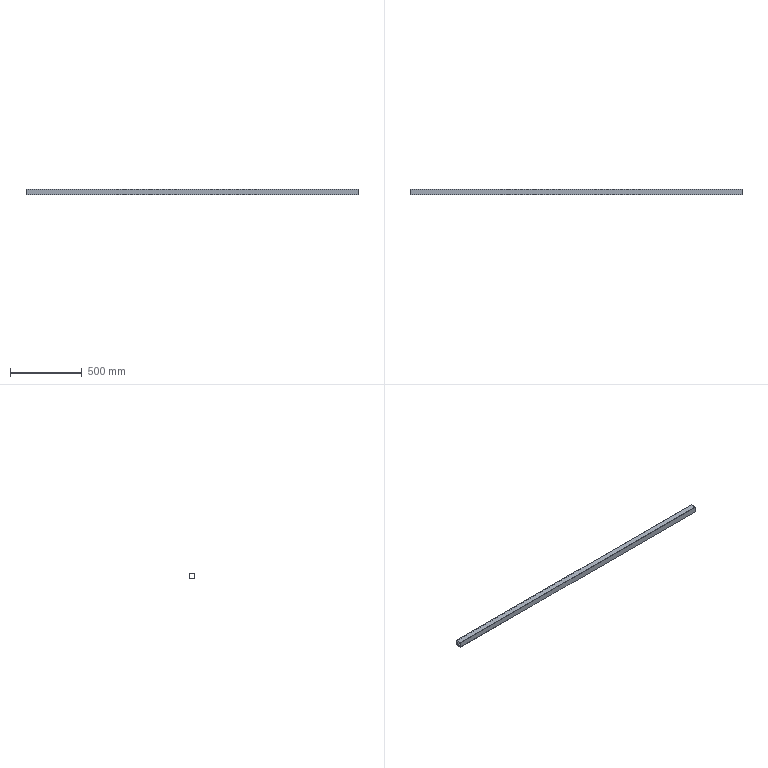Part | NX | features solid 2 | 1 solid | 10 faces | box 2320 x 40 x 40 mm | volume 1336320 mm3 | plane 10
STEP:
#1=CARTESIAN_POINT('',(-1180.,-220.,-45.));
#2=VERTEX_POINT('',#1);
#3=CARTESIAN_POINT('',(1140.,-220.,-45.));
#4=VERTEX_POINT('',#3);
#5=CARTESIAN_POINT('',(204.393,-220.,-45.));
#6=DIRECTION('',(1.,0.,0.));
#7=VECTOR('',#6,1000.);
#8=LINE('',#5,#7);
#9=EDGE_CURVE('',#2,#4,#8,.T.);
#10=ORIENTED_EDGE('',*,*,#9,.F.);
#11=CARTESIAN_POINT('',(-1180.,-220.,-85.));
#12=VERTEX_POINT('',#11);
#13=CARTESIAN_POINT('',(-1180.,-220.,-70.));
#14=DIRECTION('',(0.,0.,-1.));
#15=VECTOR('',#14,1000.);
#16=LINE('',#13,#15);
#17=EDGE_CURVE('',#2,#12,#16,.T.);
#18=ORIENTED_EDGE('',*,*,#17,.T.);
#19=CARTESIAN_POINT('',(1140.,-220.,-85.));
#20=VERTEX_POINT('',#19);
#21=CARTESIAN_POINT('',(119.393,-220.,-85.));
#22=DIRECTION('',(1.,0.,0.));
#23=VECTOR('',#22,1000.);
#24=LINE('',#21,#23);
#25=EDGE_CURVE('',#12,#20,#24,.T.);
#26=ORIENTED_EDGE('',*,*,#25,.T.);
#27=CARTESIAN_POINT('',(1140.,-220.,-70.));
#28=DIRECTION('',(0.,0.,-1.));
#29=VECTOR('',#28,1000.);
#30=LINE('',#27,#29);
#31=EDGE_CURVE('',#4,#20,#30,.T.);
#32=ORIENTED_EDGE('',*,*,#31,.F.);
#33=EDGE_LOOP('',(#10,#18,#26,#32));
#34=FACE_BOUND('',#33,.T.);
#35=CARTESIAN_POINT('',(119.393,-220.,-70.));
#36=DIRECTION('',(0.,1.,0.));
#37=DIRECTION('',(0.,0.,1.));
#38=AXIS2_PLACEMENT_3D('',#35,#36,#37);
#39=PLANE('',#38);
#40=ADVANCED_FACE('',(#34),#39,.F.);
#41=ORIENTED_EDGE('',*,*,#25,.F.);
#42=CARTESIAN_POINT('',(-1180.,-180.,-85.));
#43=VERTEX_POINT('',#42);
#44=CARTESIAN_POINT('',(-1180.,-800.,-85.));
#45=DIRECTION('',(0.,1.,0.));
#46=VECTOR('',#45,1000.);
#47=LINE('',#44,#46);
#48=EDGE_CURVE('',#12,#43,#47,.T.);
#49=ORIENTED_EDGE('',*,*,#48,.T.);
#50=CARTESIAN_POINT('',(1140.,-180.,-85.));
#51=VERTEX_POINT('',#50);
#52=CARTESIAN_POINT('',(204.393,-180.,-85.));
#53=DIRECTION('',(1.,0.,0.));
#54=VECTOR('',#53,1000.);
#55=LINE('',#52,#54);
#56=EDGE_CURVE('',#43,#51,#55,.T.);
#57=ORIENTED_EDGE('',*,*,#56,.T.);
#58=CARTESIAN_POINT('',(1140.,-800.,-85.));
#59=DIRECTION('',(0.,1.,0.));
#60=VECTOR('',#59,1000.);
#61=LINE('',#58,#60);
#62=EDGE_CURVE('',#20,#51,#61,.T.);
#63=ORIENTED_EDGE('',*,*,#62,.F.);
#64=EDGE_LOOP('',(#41,#49,#57,#63));
#65=FACE_BOUND('',#64,.T.);
#66=CARTESIAN_POINT('',(204.393,-800.,-85.));
#67=DIRECTION('',(0.,0.,1.));
#68=DIRECTION('',(0.,-1.,0.));
#69=AXIS2_PLACEMENT_3D('',#66,#67,#68);
#70=PLANE('',#69);
#71=ADVANCED_FACE('',(#65),#70,.F.);
#72=CARTESIAN_POINT('',(1140.,-180.,-45.));
#73=VERTEX_POINT('',#72);
#74=CARTESIAN_POINT('',(-1180.,-180.,-45.));
#75=VERTEX_POINT('',#74);
#76=CARTESIAN_POINT('',(204.393,-180.,-45.));
#77=DIRECTION('',(-1.,0.,0.));
#78=VECTOR('',#77,1000.);
#79=LINE('',#76,#78);
#80=EDGE_CURVE('',#73,#75,#79,.T.);
#81=ORIENTED_EDGE('',*,*,#80,.T.);
#82=CARTESIAN_POINT('',(-1180.,-840.,-45.));
#83=DIRECTION('',(0.,-1.,0.));
#84=VECTOR('',#83,1000.);
#85=LINE('',#82,#84);
#86=EDGE_CURVE('',#75,#2,#85,.T.);
#87=ORIENTED_EDGE('',*,*,#86,.T.);
#88=ORIENTED_EDGE('',*,*,#9,.T.);
#89=CARTESIAN_POINT('',(1140.,-840.,-45.));
#90=DIRECTION('',(0.,-1.,0.));
#91=VECTOR('',#90,1000.);
#92=LINE('',#89,#91);
#93=EDGE_CURVE('',#73,#4,#92,.T.);
#94=ORIENTED_EDGE('',*,*,#93,.F.);
#95=EDGE_LOOP('',(#81,#87,#88,#94));
#96=FACE_BOUND('',#95,.T.);
#97=CARTESIAN_POINT('',(204.393,-840.,-45.));
#98=DIRECTION('',(0.,0.,-1.));
#99=DIRECTION('',(0.,1.,0.));
#100=AXIS2_PLACEMENT_3D('',#97,#98,#99);
#101=PLANE('',#100);
#102=ADVANCED_FACE('',(#96),#101,.F.);
#103=ORIENTED_EDGE('',*,*,#56,.F.);
#104=CARTESIAN_POINT('',(-1180.,-180.,-40.));
#105=DIRECTION('',(0.,0.,1.));
#106=VECTOR('',#105,1000.);
#107=LINE('',#104,#106);
#108=EDGE_CURVE('',#43,#75,#107,.T.);
#109=ORIENTED_EDGE('',*,*,#108,.T.);
#110=ORIENTED_EDGE('',*,*,#80,.F.);
#111=CARTESIAN_POINT('',(1140.,-180.,-40.));
#112=DIRECTION('',(0.,0.,1.));
#113=VECTOR('',#112,1000.);
#114=LINE('',#111,#113);
#115=EDGE_CURVE('',#51,#73,#114,.T.);
#116=ORIENTED_EDGE('',*,*,#115,.F.);
#117=EDGE_LOOP('',(#103,#109,#110,#116));
#118=FACE_BOUND('',#117,.T.);
#119=CARTESIAN_POINT('',(119.393,-180.,-40.));
#120=DIRECTION('',(0.,-1.,0.));
#121=DIRECTION('',(0.,0.,-1.));
#122=AXIS2_PLACEMENT_3D('',#119,#120,#121);
#123=PLANE('',#122);
#124=ADVANCED_FACE('',(#118),#123,.F.);
#125=CARTESIAN_POINT('',(-1180.,-216.,-49.));
#126=VERTEX_POINT('',#125);
#127=CARTESIAN_POINT('',(-1180.,-216.,-81.));
#128=VERTEX_POINT('',#127);
#129=CARTESIAN_POINT('',(-1180.,-216.,-70.));
#130=DIRECTION('',(0.,0.,-1.));
#131=VECTOR('',#130,1000.);
#132=LINE('',#129,#131);
#133=EDGE_CURVE('',#126,#128,#132,.T.);
#134=ORIENTED_EDGE('',*,*,#133,.F.);
#135=CARTESIAN_POINT('',(1140.,-216.,-49.));
#136=VERTEX_POINT('',#135);
#137=CARTESIAN_POINT('',(204.393,-216.,-49.));
#138=DIRECTION('',(1.,0.,0.));
#139=VECTOR('',#138,1000.);
#140=LINE('',#137,#139);
#141=EDGE_CURVE('',#126,#136,#140,.T.);
#142=ORIENTED_EDGE('',*,*,#141,.T.);
#143=CARTESIAN_POINT('',(1140.,-216.,-81.));
#144=VERTEX_POINT('',#143);
#145=CARTESIAN_POINT('',(1140.,-216.,-70.));
#146=DIRECTION('',(0.,0.,-1.));
#147=VECTOR('',#146,1000.);
#148=LINE('',#145,#147);
#149=EDGE_CURVE('',#136,#144,#148,.T.);
#150=ORIENTED_EDGE('',*,*,#149,.T.);
#151=CARTESIAN_POINT('',(119.393,-216.,-81.));
#152=DIRECTION('',(1.,0.,0.));
#153=VECTOR('',#152,1000.);
#154=LINE('',#151,#153);
#155=EDGE_CURVE('',#128,#144,#154,.T.);
#156=ORIENTED_EDGE('',*,*,#155,.F.);
#157=EDGE_LOOP('',(#134,#142,#150,#156));
#158=FACE_BOUND('',#157,.T.);
#159=CARTESIAN_POINT('',(119.393,-216.,-70.));
#160=DIRECTION('',(0.,1.,0.));
#161=DIRECTION('',(0.,0.,1.));
#162=AXIS2_PLACEMENT_3D('',#159,#160,#161);
#163=PLANE('',#162);
#164=ADVANCED_FACE('',(#158),#163,.T.);
#165=CARTESIAN_POINT('',(-1180.,-184.,-81.));
#166=VERTEX_POINT('',#165);
#167=CARTESIAN_POINT('',(-1180.,-800.,-81.));
#168=DIRECTION('',(0.,1.,0.));
#169=VECTOR('',#168,1000.);
#170=LINE('',#167,#169);
#171=EDGE_CURVE('',#128,#166,#170,.T.);
#172=ORIENTED_EDGE('',*,*,#171,.F.);
#173=ORIENTED_EDGE('',*,*,#155,.T.);
#174=CARTESIAN_POINT('',(1140.,-184.,-81.));
#175=VERTEX_POINT('',#174);
#176=CARTESIAN_POINT('',(1140.,-800.,-81.));
#177=DIRECTION('',(0.,1.,0.));
#178=VECTOR('',#177,1000.);
#179=LINE('',#176,#178);
#180=EDGE_CURVE('',#144,#175,#179,.T.);
#181=ORIENTED_EDGE('',*,*,#180,.T.);
#182=CARTESIAN_POINT('',(204.393,-184.,-81.));
#183=DIRECTION('',(1.,0.,0.));
#184=VECTOR('',#183,1000.);
#185=LINE('',#182,#184);
#186=EDGE_CURVE('',#166,#175,#185,.T.);
#187=ORIENTED_EDGE('',*,*,#186,.F.);
#188=EDGE_LOOP('',(#172,#173,#181,#187));
#189=FACE_BOUND('',#188,.T.);
#190=CARTESIAN_POINT('',(204.393,-800.,-81.));
#191=DIRECTION('',(0.,0.,1.));
#192=DIRECTION('',(0.,-1.,0.));
#193=AXIS2_PLACEMENT_3D('',#190,#191,#192);
#194=PLANE('',#193);
#195=ADVANCED_FACE('',(#189),#194,.T.);
#196=CARTESIAN_POINT('',(-1180.,-184.,-49.));
#197=VERTEX_POINT('',#196);
#198=CARTESIAN_POINT('',(-1180.,-840.,-49.));
#199=DIRECTION('',(0.,-1.,0.));
#200=VECTOR('',#199,1000.);
#201=LINE('',#198,#200);
#202=EDGE_CURVE('',#197,#126,#201,.T.);
#203=ORIENTED_EDGE('',*,*,#202,.F.);
#204=CARTESIAN_POINT('',(1140.,-184.,-49.));
#205=VERTEX_POINT('',#204);
#206=CARTESIAN_POINT('',(204.393,-184.,-49.));
#207=DIRECTION('',(-1.,0.,0.));
#208=VECTOR('',#207,1000.);
#209=LINE('',#206,#208);
#210=EDGE_CURVE('',#205,#197,#209,.T.);
#211=ORIENTED_EDGE('',*,*,#210,.F.);
#212=CARTESIAN_POINT('',(1140.,-840.,-49.));
#213=DIRECTION('',(0.,-1.,0.));
#214=VECTOR('',#213,1000.);
#215=LINE('',#212,#214);
#216=EDGE_CURVE('',#205,#136,#215,.T.);
#217=ORIENTED_EDGE('',*,*,#216,.T.);
#218=ORIENTED_EDGE('',*,*,#141,.F.);
#219=EDGE_LOOP('',(#203,#211,#217,#218));
#220=FACE_BOUND('',#219,.T.);
#221=CARTESIAN_POINT('',(204.393,-840.,-49.));
#222=DIRECTION('',(0.,0.,-1.));
#223=DIRECTION('',(0.,1.,0.));
#224=AXIS2_PLACEMENT_3D('',#221,#222,#223);
#225=PLANE('',#224);
#226=ADVANCED_FACE('',(#220),#225,.T.);
#227=CARTESIAN_POINT('',(-1180.,-184.,-40.));
#228=DIRECTION('',(0.,0.,1.));
#229=VECTOR('',#228,1000.);
#230=LINE('',#227,#229);
#231=EDGE_CURVE('',#166,#197,#230,.T.);
#232=ORIENTED_EDGE('',*,*,#231,.F.);
#233=ORIENTED_EDGE('',*,*,#186,.T.);
#234=CARTESIAN_POINT('',(1140.,-184.,-40.));
#235=DIRECTION('',(0.,0.,1.));
#236=VECTOR('',#235,1000.);
#237=LINE('',#234,#236);
#238=EDGE_CURVE('',#175,#205,#237,.T.);
#239=ORIENTED_EDGE('',*,*,#238,.T.);
#240=ORIENTED_EDGE('',*,*,#210,.T.);
#241=EDGE_LOOP('',(#232,#233,#239,#240));
#242=FACE_BOUND('',#241,.T.);
#243=CARTESIAN_POINT('',(119.393,-184.,-40.));
#244=DIRECTION('',(0.,-1.,0.));
#245=DIRECTION('',(0.,0.,-1.));
#246=AXIS2_PLACEMENT_3D('',#243,#244,#245);
#247=PLANE('',#246);
#248=ADVANCED_FACE('',(#242),#247,.T.);
#249=ORIENTED_EDGE('',*,*,#149,.F.);
#250=ORIENTED_EDGE('',*,*,#216,.F.);
#251=ORIENTED_EDGE('',*,*,#238,.F.);
#252=ORIENTED_EDGE('',*,*,#180,.F.);
#253=EDGE_LOOP('',(#249,#250,#251,#252));
#254=FACE_BOUND('',#253,.T.);
#255=ORIENTED_EDGE('',*,*,#93,.T.);
#256=ORIENTED_EDGE('',*,*,#31,.T.);
#257=ORIENTED_EDGE('',*,*,#62,.T.);
#258=ORIENTED_EDGE('',*,*,#115,.T.);
#259=EDGE_LOOP('',(#255,#256,#257,#258));
#260=FACE_BOUND('',#259,.T.);
#261=CARTESIAN_POINT('',(1140.,-247.5,-9.5));
#262=DIRECTION('',(1.,0.,0.));
#263=DIRECTION('',(0.,0.,-1.));
#264=AXIS2_PLACEMENT_3D('',#261,#262,#263);
#265=PLANE('',#264);
#266=ADVANCED_FACE('',(#254,#260),#265,.T.);
#267=ORIENTED_EDGE('',*,*,#133,.T.);
#268=ORIENTED_EDGE('',*,*,#171,.T.);
#269=ORIENTED_EDGE('',*,*,#231,.T.);
#270=ORIENTED_EDGE('',*,*,#202,.T.);
#271=EDGE_LOOP('',(#267,#268,#269,#270));
#272=FACE_BOUND('',#271,.T.);
#273=ORIENTED_EDGE('',*,*,#86,.F.);
#274=ORIENTED_EDGE('',*,*,#108,.F.);
#275=ORIENTED_EDGE('',*,*,#48,.F.);
#276=ORIENTED_EDGE('',*,*,#17,.F.);
#277=EDGE_LOOP('',(#273,#274,#275,#276));
#278=FACE_BOUND('',#277,.T.);
#279=CARTESIAN_POINT('',(-1180.,-180.,-45.));
#280=DIRECTION('',(1.,0.,0.));
#281=DIRECTION('',(0.,0.,-1.));
#282=AXIS2_PLACEMENT_3D('',#279,#280,#281);
#283=PLANE('',#282);
#284=ADVANCED_FACE('',(#272,#278),#283,.F.);
#285=CLOSED_SHELL('',(#40,#71,#102,#124,#164,#195,#226,#248,#266,#284));
#286=MANIFOLD_SOLID_BREP('',#285);
#287=(LENGTH_UNIT()NAMED_UNIT(*)SI_UNIT(.MILLI.,.METRE.));
#288=UNCERTAINTY_MEASURE_WITH_UNIT(LENGTH_MEASURE(0.00001),#287,'','');
#289=(NAMED_UNIT(*)PLANE_ANGLE_UNIT()SI_UNIT($,.RADIAN.));
#290=(NAMED_UNIT(*)SI_UNIT($,.STERADIAN.)SOLID_ANGLE_UNIT());
#291=(GEOMETRIC_REPRESENTATION_CONTEXT(3)GLOBAL_UNCERTAINTY_ASSIGNED_CONTEXT((#288))GLOBAL_UNIT_ASSIGNED_CONTEXT((#287,#289,#290))REPRESENTATION_CONTEXT('',''));
#292=ADVANCED_BREP_SHAPE_REPRESENTATION('',(#286),#291);